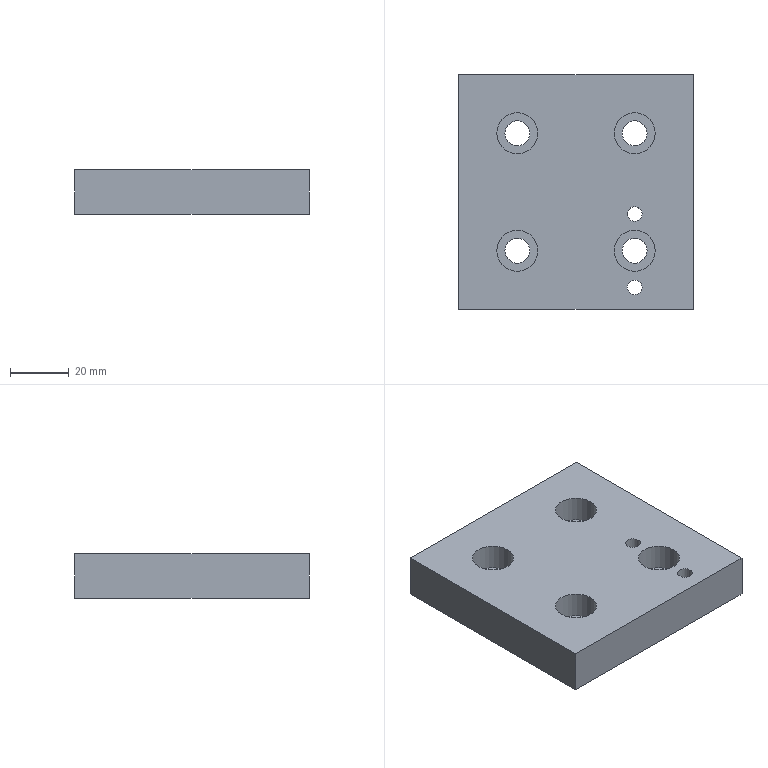Part | STEP file | 1 solid | 20 faces | box 80 x 80 x 15 mm | volume 88507 mm3 | plane 10 | cylinder 10 | commonest cylinder face diameters 8.5 x4 14 x4 5 x2
STEP:
#1=CARTESIAN_POINT('',(0.,0.,0.));
#2=DIRECTION('',(0.,0.,1.));
#3=DIRECTION('',(1.,0.,0.));
#4=AXIS2_PLACEMENT_3D('',#1,#2,#3);
#5=CARTESIAN_POINT('',(-5.75,-35.432,0.));
#6=VERTEX_POINT('',#5);
#7=CARTESIAN_POINT('',(-10.,-35.432,0.));
#8=DIRECTION('',(0.,0.,-1.));
#9=DIRECTION('',(1.,0.,0.));
#10=AXIS2_PLACEMENT_3D('',#7,#8,#9);
#11=CIRCLE('',#10,4.25);
#12=CARTESIAN_POINT('',(0.,0.,0.));
#13=DIRECTION('',(0.,0.,1.));
#14=DIRECTION('',(1.,0.,0.));
#15=AXIS2_PLACEMENT_3D('',#12,#13,#14);
#16=PLANE('',#15);
#17=CARTESIAN_POINT('',(-5.75,-35.432));
#18=CARTESIAN_POINT('',(-5.75,-42.793));
#19=CARTESIAN_POINT('',(-12.125,-39.113));
#20=CARTESIAN_POINT('',(-18.5,-35.432));
#21=CARTESIAN_POINT('',(-12.125,-31.751));
#22=CARTESIAN_POINT('',(-5.75,-28.071));
#23=CARTESIAN_POINT('',(-5.75,-35.432));
#24=(BOUNDED_CURVE()B_SPLINE_CURVE(2,(#17,#18,#19,#20,#21,#22,#23),.UNSPECIFIED.,.T.,.F.)B_SPLINE_CURVE_WITH_KNOTS((1,2,2,2,2,1),(-2.094,0.,2.094,4.189,6.283,8.378),.UNSPECIFIED.)CURVE()GEOMETRIC_REPRESENTATION_ITEM()RATIONAL_B_SPLINE_CURVE((1.,0.5,1.,0.5,1.,0.5,1.))REPRESENTATION_ITEM(''));
#25=(GEOMETRIC_REPRESENTATION_CONTEXT(2)PARAMETRIC_REPRESENTATION_CONTEXT()REPRESENTATION_CONTEXT('',''));
#26=DEFINITIONAL_REPRESENTATION('',(#24),#25);
#27=PCURVE('',#16,#26);
#28=CARTESIAN_POINT('',(-10.,-35.432,15.));
#29=DIRECTION('',(0.,0.,1.));
#30=DIRECTION('',(1.,0.,0.));
#31=AXIS2_PLACEMENT_3D('',#28,#29,#30);
#32=CYLINDRICAL_SURFACE('',#31,4.25);
#33=CARTESIAN_POINT('',(6.283,-15.));
#34=DIRECTION('',(-1.,0.));
#35=VECTOR('',#34,1.);
#36=LINE('',#33,#35);
#37=(GEOMETRIC_REPRESENTATION_CONTEXT(2)PARAMETRIC_REPRESENTATION_CONTEXT()REPRESENTATION_CONTEXT('',''));
#38=DEFINITIONAL_REPRESENTATION('',(#36),#37);
#39=PCURVE('',#32,#38);
#40=SURFACE_CURVE('',#11,(#27,#39),.PCURVE_S1.);
#41=EDGE_CURVE('',#6,#6,#40,.T.);
#42=ORIENTED_EDGE('',*,*,#41,.F.);
#43=EDGE_LOOP('',(#42));
#44=FACE_BOUND('',#43,.T.);
#45=CARTESIAN_POINT('',(-45.75,-35.432,0.));
#46=VERTEX_POINT('',#45);
#47=CARTESIAN_POINT('',(-50.,-35.432,0.));
#48=DIRECTION('',(0.,0.,-1.));
#49=DIRECTION('',(1.,0.,0.));
#50=AXIS2_PLACEMENT_3D('',#47,#48,#49);
#51=CIRCLE('',#50,4.25);
#52=CARTESIAN_POINT('',(-45.75,-35.432));
#53=CARTESIAN_POINT('',(-45.75,-42.793));
#54=CARTESIAN_POINT('',(-52.125,-39.113));
#55=CARTESIAN_POINT('',(-58.5,-35.432));
#56=CARTESIAN_POINT('',(-52.125,-31.751));
#57=CARTESIAN_POINT('',(-45.75,-28.071));
#58=CARTESIAN_POINT('',(-45.75,-35.432));
#59=(BOUNDED_CURVE()B_SPLINE_CURVE(2,(#52,#53,#54,#55,#56,#57,#58),.UNSPECIFIED.,.T.,.F.)B_SPLINE_CURVE_WITH_KNOTS((1,2,2,2,2,1),(-2.094,0.,2.094,4.189,6.283,8.378),.UNSPECIFIED.)CURVE()GEOMETRIC_REPRESENTATION_ITEM()RATIONAL_B_SPLINE_CURVE((1.,0.5,1.,0.5,1.,0.5,1.))REPRESENTATION_ITEM(''));
#60=(GEOMETRIC_REPRESENTATION_CONTEXT(2)PARAMETRIC_REPRESENTATION_CONTEXT()REPRESENTATION_CONTEXT('',''));
#61=DEFINITIONAL_REPRESENTATION('',(#59),#60);
#62=PCURVE('',#16,#61);
#63=CARTESIAN_POINT('',(-50.,-35.432,15.));
#64=DIRECTION('',(0.,0.,1.));
#65=DIRECTION('',(1.,0.,0.));
#66=AXIS2_PLACEMENT_3D('',#63,#64,#65);
#67=CYLINDRICAL_SURFACE('',#66,4.25);
#68=CARTESIAN_POINT('',(6.283,-15.));
#69=DIRECTION('',(-1.,0.));
#70=VECTOR('',#69,1.);
#71=LINE('',#68,#70);
#72=(GEOMETRIC_REPRESENTATION_CONTEXT(2)PARAMETRIC_REPRESENTATION_CONTEXT()REPRESENTATION_CONTEXT('',''));
#73=DEFINITIONAL_REPRESENTATION('',(#71),#72);
#74=PCURVE('',#67,#73);
#75=SURFACE_CURVE('',#51,(#62,#74),.PCURVE_S1.);
#76=EDGE_CURVE('',#46,#46,#75,.T.);
#77=ORIENTED_EDGE('',*,*,#76,.F.);
#78=EDGE_LOOP('',(#77));
#79=FACE_BOUND('',#78,.T.);
#80=CARTESIAN_POINT('',(-45.75,4.568,0.));
#81=VERTEX_POINT('',#80);
#82=CARTESIAN_POINT('',(-50.,4.568,0.));
#83=DIRECTION('',(0.,0.,-1.));
#84=DIRECTION('',(1.,0.,0.));
#85=AXIS2_PLACEMENT_3D('',#82,#83,#84);
#86=CIRCLE('',#85,4.25);
#87=CARTESIAN_POINT('',(-45.75,4.568));
#88=CARTESIAN_POINT('',(-45.75,-2.793));
#89=CARTESIAN_POINT('',(-52.125,0.8873));
#90=CARTESIAN_POINT('',(-58.5,4.568));
#91=CARTESIAN_POINT('',(-52.125,8.249));
#92=CARTESIAN_POINT('',(-45.75,11.929));
#93=CARTESIAN_POINT('',(-45.75,4.568));
#94=(BOUNDED_CURVE()B_SPLINE_CURVE(2,(#87,#88,#89,#90,#91,#92,#93),.UNSPECIFIED.,.T.,.F.)B_SPLINE_CURVE_WITH_KNOTS((1,2,2,2,2,1),(-2.094,0.,2.094,4.189,6.283,8.378),.UNSPECIFIED.)CURVE()GEOMETRIC_REPRESENTATION_ITEM()RATIONAL_B_SPLINE_CURVE((1.,0.5,1.,0.5,1.,0.5,1.))REPRESENTATION_ITEM(''));
#95=(GEOMETRIC_REPRESENTATION_CONTEXT(2)PARAMETRIC_REPRESENTATION_CONTEXT()REPRESENTATION_CONTEXT('',''));
#96=DEFINITIONAL_REPRESENTATION('',(#94),#95);
#97=PCURVE('',#16,#96);
#98=CARTESIAN_POINT('',(-50.,4.568,15.));
#99=DIRECTION('',(0.,0.,1.));
#100=DIRECTION('',(1.,0.,0.));
#101=AXIS2_PLACEMENT_3D('',#98,#99,#100);
#102=CYLINDRICAL_SURFACE('',#101,4.25);
#103=CARTESIAN_POINT('',(6.283,-15.));
#104=DIRECTION('',(-1.,0.));
#105=VECTOR('',#104,1.);
#106=LINE('',#103,#105);
#107=(GEOMETRIC_REPRESENTATION_CONTEXT(2)PARAMETRIC_REPRESENTATION_CONTEXT()REPRESENTATION_CONTEXT('',''));
#108=DEFINITIONAL_REPRESENTATION('',(#106),#107);
#109=PCURVE('',#102,#108);
#110=SURFACE_CURVE('',#86,(#97,#109),.PCURVE_S1.);
#111=EDGE_CURVE('',#81,#81,#110,.T.);
#112=ORIENTED_EDGE('',*,*,#111,.F.);
#113=EDGE_LOOP('',(#112));
#114=FACE_BOUND('',#113,.T.);
#115=CARTESIAN_POINT('',(-5.75,4.568,0.));
#116=VERTEX_POINT('',#115);
#117=CARTESIAN_POINT('',(-10.,4.568,0.));
#118=DIRECTION('',(0.,0.,-1.));
#119=DIRECTION('',(1.,0.,0.));
#120=AXIS2_PLACEMENT_3D('',#117,#118,#119);
#121=CIRCLE('',#120,4.25);
#122=CARTESIAN_POINT('',(-5.75,4.568));
#123=CARTESIAN_POINT('',(-5.75,-2.793));
#124=CARTESIAN_POINT('',(-12.125,0.8873));
#125=CARTESIAN_POINT('',(-18.5,4.568));
#126=CARTESIAN_POINT('',(-12.125,8.249));
#127=CARTESIAN_POINT('',(-5.75,11.929));
#128=CARTESIAN_POINT('',(-5.75,4.568));
#129=(BOUNDED_CURVE()B_SPLINE_CURVE(2,(#122,#123,#124,#125,#126,#127,#128),.UNSPECIFIED.,.T.,.F.)B_SPLINE_CURVE_WITH_KNOTS((1,2,2,2,2,1),(-2.094,0.,2.094,4.189,6.283,8.378),.UNSPECIFIED.)CURVE()GEOMETRIC_REPRESENTATION_ITEM()RATIONAL_B_SPLINE_CURVE((1.,0.5,1.,0.5,1.,0.5,1.))REPRESENTATION_ITEM(''));
#130=(GEOMETRIC_REPRESENTATION_CONTEXT(2)PARAMETRIC_REPRESENTATION_CONTEXT()REPRESENTATION_CONTEXT('',''));
#131=DEFINITIONAL_REPRESENTATION('',(#129),#130);
#132=PCURVE('',#16,#131);
#133=CARTESIAN_POINT('',(-10.,4.568,15.));
#134=DIRECTION('',(0.,0.,1.));
#135=DIRECTION('',(1.,0.,0.));
#136=AXIS2_PLACEMENT_3D('',#133,#134,#135);
#137=CYLINDRICAL_SURFACE('',#136,4.25);
#138=CARTESIAN_POINT('',(6.283,-15.));
#139=DIRECTION('',(-1.,0.));
#140=VECTOR('',#139,1.);
#141=LINE('',#138,#140);
#142=(GEOMETRIC_REPRESENTATION_CONTEXT(2)PARAMETRIC_REPRESENTATION_CONTEXT()REPRESENTATION_CONTEXT('',''));
#143=DEFINITIONAL_REPRESENTATION('',(#141),#142);
#144=PCURVE('',#137,#143);
#145=SURFACE_CURVE('',#121,(#132,#144),.PCURVE_S1.);
#146=EDGE_CURVE('',#116,#116,#145,.T.);
#147=ORIENTED_EDGE('',*,*,#146,.F.);
#148=EDGE_LOOP('',(#147));
#149=FACE_BOUND('',#148,.T.);
#150=CARTESIAN_POINT('',(-7.5,-47.932,0.));
#151=VERTEX_POINT('',#150);
#152=CARTESIAN_POINT('',(-10.,-47.932,0.));
#153=DIRECTION('',(0.,0.,-1.));
#154=DIRECTION('',(1.,0.,0.));
#155=AXIS2_PLACEMENT_3D('',#152,#153,#154);
#156=CIRCLE('',#155,2.5);
#157=CARTESIAN_POINT('',(-7.5,-47.932));
#158=CARTESIAN_POINT('',(-7.5,-52.262));
#159=CARTESIAN_POINT('',(-11.25,-50.097));
#160=CARTESIAN_POINT('',(-15.,-47.932));
#161=CARTESIAN_POINT('',(-11.25,-45.767));
#162=CARTESIAN_POINT('',(-7.5,-43.602));
#163=CARTESIAN_POINT('',(-7.5,-47.932));
#164=(BOUNDED_CURVE()B_SPLINE_CURVE(2,(#157,#158,#159,#160,#161,#162,#163),.UNSPECIFIED.,.T.,.F.)B_SPLINE_CURVE_WITH_KNOTS((1,2,2,2,2,1),(-2.094,0.,2.094,4.189,6.283,8.378),.UNSPECIFIED.)CURVE()GEOMETRIC_REPRESENTATION_ITEM()RATIONAL_B_SPLINE_CURVE((1.,0.5,1.,0.5,1.,0.5,1.))REPRESENTATION_ITEM(''));
#165=(GEOMETRIC_REPRESENTATION_CONTEXT(2)PARAMETRIC_REPRESENTATION_CONTEXT()REPRESENTATION_CONTEXT('',''));
#166=DEFINITIONAL_REPRESENTATION('',(#164),#165);
#167=PCURVE('',#16,#166);
#168=CARTESIAN_POINT('',(-10.,-47.932,15.));
#169=DIRECTION('',(0.,0.,1.));
#170=DIRECTION('',(1.,0.,0.));
#171=AXIS2_PLACEMENT_3D('',#168,#169,#170);
#172=CYLINDRICAL_SURFACE('',#171,2.5);
#173=CARTESIAN_POINT('',(6.283,-15.));
#174=DIRECTION('',(-1.,0.));
#175=VECTOR('',#174,1.);
#176=LINE('',#173,#175);
#177=(GEOMETRIC_REPRESENTATION_CONTEXT(2)PARAMETRIC_REPRESENTATION_CONTEXT()REPRESENTATION_CONTEXT('',''));
#178=DEFINITIONAL_REPRESENTATION('',(#176),#177);
#179=PCURVE('',#172,#178);
#180=SURFACE_CURVE('',#156,(#167,#179),.PCURVE_S1.);
#181=EDGE_CURVE('',#151,#151,#180,.T.);
#182=ORIENTED_EDGE('',*,*,#181,.F.);
#183=EDGE_LOOP('',(#182));
#184=FACE_BOUND('',#183,.T.);
#185=CARTESIAN_POINT('',(-7.5,-22.932,0.));
#186=VERTEX_POINT('',#185);
#187=CARTESIAN_POINT('',(-10.,-22.932,0.));
#188=DIRECTION('',(0.,0.,-1.));
#189=DIRECTION('',(1.,0.,0.));
#190=AXIS2_PLACEMENT_3D('',#187,#188,#189);
#191=CIRCLE('',#190,2.5);
#192=CARTESIAN_POINT('',(-7.5,-22.932));
#193=CARTESIAN_POINT('',(-7.5,-27.262));
#194=CARTESIAN_POINT('',(-11.25,-25.097));
#195=CARTESIAN_POINT('',(-15.,-22.932));
#196=CARTESIAN_POINT('',(-11.25,-20.767));
#197=CARTESIAN_POINT('',(-7.5,-18.602));
#198=CARTESIAN_POINT('',(-7.5,-22.932));
#199=(BOUNDED_CURVE()B_SPLINE_CURVE(2,(#192,#193,#194,#195,#196,#197,#198),.UNSPECIFIED.,.T.,.F.)B_SPLINE_CURVE_WITH_KNOTS((1,2,2,2,2,1),(-2.094,0.,2.094,4.189,6.283,8.378),.UNSPECIFIED.)CURVE()GEOMETRIC_REPRESENTATION_ITEM()RATIONAL_B_SPLINE_CURVE((1.,0.5,1.,0.5,1.,0.5,1.))REPRESENTATION_ITEM(''));
#200=(GEOMETRIC_REPRESENTATION_CONTEXT(2)PARAMETRIC_REPRESENTATION_CONTEXT()REPRESENTATION_CONTEXT('',''));
#201=DEFINITIONAL_REPRESENTATION('',(#199),#200);
#202=PCURVE('',#16,#201);
#203=CARTESIAN_POINT('',(-10.,-22.932,15.));
#204=DIRECTION('',(0.,0.,1.));
#205=DIRECTION('',(1.,0.,0.));
#206=AXIS2_PLACEMENT_3D('',#203,#204,#205);
#207=CYLINDRICAL_SURFACE('',#206,2.5);
#208=CARTESIAN_POINT('',(6.283,-15.));
#209=DIRECTION('',(-1.,0.));
#210=VECTOR('',#209,1.);
#211=LINE('',#208,#210);
#212=(GEOMETRIC_REPRESENTATION_CONTEXT(2)PARAMETRIC_REPRESENTATION_CONTEXT()REPRESENTATION_CONTEXT('',''));
#213=DEFINITIONAL_REPRESENTATION('',(#211),#212);
#214=PCURVE('',#207,#213);
#215=SURFACE_CURVE('',#191,(#202,#214),.PCURVE_S1.);
#216=EDGE_CURVE('',#186,#186,#215,.T.);
#217=ORIENTED_EDGE('',*,*,#216,.F.);
#218=EDGE_LOOP('',(#217));
#219=FACE_BOUND('',#218,.T.);
#220=CARTESIAN_POINT('',(10.,24.568,0.));
#221=VERTEX_POINT('',#220);
#222=CARTESIAN_POINT('',(-70.,24.568,0.));
#223=VERTEX_POINT('',#222);
#224=CARTESIAN_POINT('',(0.,24.568,0.));
#225=DIRECTION('',(-1.,0.,0.));
#226=VECTOR('',#225,1.);
#227=LINE('',#224,#226);
#228=CARTESIAN_POINT('',(0.,24.568));
#229=DIRECTION('',(-1.,0.));
#230=VECTOR('',#229,1.);
#231=LINE('',#228,#230);
#232=(GEOMETRIC_REPRESENTATION_CONTEXT(2)PARAMETRIC_REPRESENTATION_CONTEXT()REPRESENTATION_CONTEXT('',''));
#233=DEFINITIONAL_REPRESENTATION('',(#231),#232);
#234=PCURVE('',#16,#233);
#235=CARTESIAN_POINT('',(-70.,24.568,15.));
#236=DIRECTION('',(0.,-1.,0.));
#237=DIRECTION('',(0.,0.,-1.));
#238=AXIS2_PLACEMENT_3D('',#235,#236,#237);
#239=PLANE('',#238);
#240=CARTESIAN_POINT('',(15.,70.));
#241=DIRECTION('',(0.,-1.));
#242=VECTOR('',#241,1.);
#243=LINE('',#240,#242);
#244=(GEOMETRIC_REPRESENTATION_CONTEXT(2)PARAMETRIC_REPRESENTATION_CONTEXT()REPRESENTATION_CONTEXT('',''));
#245=DEFINITIONAL_REPRESENTATION('',(#243),#244);
#246=PCURVE('',#239,#245);
#247=SURFACE_CURVE('',#227,(#234,#246),.PCURVE_S1.);
#248=EDGE_CURVE('',#221,#223,#247,.T.);
#249=ORIENTED_EDGE('',*,*,#248,.F.);
#250=CARTESIAN_POINT('',(10.,-55.432,0.));
#251=VERTEX_POINT('',#250);
#252=CARTESIAN_POINT('',(10.,0.,0.));
#253=DIRECTION('',(0.,1.,0.));
#254=VECTOR('',#253,1.);
#255=LINE('',#252,#254);
#256=CARTESIAN_POINT('',(10.,0.));
#257=DIRECTION('',(0.,1.));
#258=VECTOR('',#257,1.);
#259=LINE('',#256,#258);
#260=(GEOMETRIC_REPRESENTATION_CONTEXT(2)PARAMETRIC_REPRESENTATION_CONTEXT()REPRESENTATION_CONTEXT('',''));
#261=DEFINITIONAL_REPRESENTATION('',(#259),#260);
#262=PCURVE('',#16,#261);
#263=CARTESIAN_POINT('',(10.,24.568,15.));
#264=DIRECTION('',(-1.,0.,0.));
#265=DIRECTION('',(0.,-1.,0.));
#266=AXIS2_PLACEMENT_3D('',#263,#264,#265);
#267=PLANE('',#266);
#268=CARTESIAN_POINT('',(24.568,-15.));
#269=DIRECTION('',(-1.,0.));
#270=VECTOR('',#269,1.);
#271=LINE('',#268,#270);
#272=(GEOMETRIC_REPRESENTATION_CONTEXT(2)PARAMETRIC_REPRESENTATION_CONTEXT()REPRESENTATION_CONTEXT('',''));
#273=DEFINITIONAL_REPRESENTATION('',(#271),#272);
#274=PCURVE('',#267,#273);
#275=SURFACE_CURVE('',#255,(#262,#274),.PCURVE_S1.);
#276=EDGE_CURVE('',#251,#221,#275,.T.);
#277=ORIENTED_EDGE('',*,*,#276,.F.);
#278=CARTESIAN_POINT('',(-70.,-55.432,0.));
#279=VERTEX_POINT('',#278);
#280=CARTESIAN_POINT('',(0.,-55.432,0.));
#281=DIRECTION('',(1.,0.,0.));
#282=VECTOR('',#281,1.);
#283=LINE('',#280,#282);
#284=CARTESIAN_POINT('',(0.,-55.432));
#285=DIRECTION('',(1.,0.));
#286=VECTOR('',#285,1.);
#287=LINE('',#284,#286);
#288=(GEOMETRIC_REPRESENTATION_CONTEXT(2)PARAMETRIC_REPRESENTATION_CONTEXT()REPRESENTATION_CONTEXT('',''));
#289=DEFINITIONAL_REPRESENTATION('',(#287),#288);
#290=PCURVE('',#16,#289);
#291=CARTESIAN_POINT('',(-70.,-55.432,15.));
#292=DIRECTION('',(0.,1.,0.));
#293=DIRECTION('',(0.,0.,1.));
#294=AXIS2_PLACEMENT_3D('',#291,#292,#293);
#295=PLANE('',#294);
#296=CARTESIAN_POINT('',(-15.,70.));
#297=DIRECTION('',(0.,1.));
#298=VECTOR('',#297,1.);
#299=LINE('',#296,#298);
#300=(GEOMETRIC_REPRESENTATION_CONTEXT(2)PARAMETRIC_REPRESENTATION_CONTEXT()REPRESENTATION_CONTEXT('',''));
#301=DEFINITIONAL_REPRESENTATION('',(#299),#300);
#302=PCURVE('',#295,#301);
#303=SURFACE_CURVE('',#283,(#290,#302),.PCURVE_S1.);
#304=EDGE_CURVE('',#279,#251,#303,.T.);
#305=ORIENTED_EDGE('',*,*,#304,.F.);
#306=CARTESIAN_POINT('',(-70.,0.,0.));
#307=DIRECTION('',(0.,-1.,0.));
#308=VECTOR('',#307,1.);
#309=LINE('',#306,#308);
#310=CARTESIAN_POINT('',(-70.,0.));
#311=DIRECTION('',(0.,-1.));
#312=VECTOR('',#311,1.);
#313=LINE('',#310,#312);
#314=(GEOMETRIC_REPRESENTATION_CONTEXT(2)PARAMETRIC_REPRESENTATION_CONTEXT()REPRESENTATION_CONTEXT('',''));
#315=DEFINITIONAL_REPRESENTATION('',(#313),#314);
#316=PCURVE('',#16,#315);
#317=CARTESIAN_POINT('',(-70.,24.568,15.));
#318=DIRECTION('',(1.,0.,0.));
#319=DIRECTION('',(0.,0.,-1.));
#320=AXIS2_PLACEMENT_3D('',#317,#318,#319);
#321=PLANE('',#320);
#322=CARTESIAN_POINT('',(15.,-24.568));
#323=DIRECTION('',(0.,-1.));
#324=VECTOR('',#323,1.);
#325=LINE('',#322,#324);
#326=(GEOMETRIC_REPRESENTATION_CONTEXT(2)PARAMETRIC_REPRESENTATION_CONTEXT()REPRESENTATION_CONTEXT('',''));
#327=DEFINITIONAL_REPRESENTATION('',(#325),#326);
#328=PCURVE('',#321,#327);
#329=SURFACE_CURVE('',#309,(#316,#328),.PCURVE_S1.);
#330=EDGE_CURVE('',#223,#279,#329,.T.);
#331=ORIENTED_EDGE('',*,*,#330,.F.);
#332=EDGE_LOOP('',(#249,#277,#305,#331));
#333=FACE_BOUND('',#332,.T.);
#334=ADVANCED_FACE('',(#44,#79,#114,#149,#184,#219,#333),#16,.F.);
#335=ORIENTED_EDGE('',*,*,#41,.F.);
#336=CARTESIAN_POINT('',(-5.75,-35.432,6.));
#337=VERTEX_POINT('',#336);
#338=CARTESIAN_POINT('',(-5.75,-35.432,0.));
#339=CARTESIAN_POINT('',(-5.75,-35.432,6.));
#340=B_SPLINE_CURVE_WITH_KNOTS('',1,(#338,#339),.UNSPECIFIED.,.F.,.F.,(2,2),(-15.,-9.),.PIECEWISE_BEZIER_KNOTS.);
#341=CARTESIAN_POINT('',(6.283,0.));
#342=DIRECTION('',(0.,1.));
#343=VECTOR('',#342,1.);
#344=LINE('',#341,#343);
#345=(GEOMETRIC_REPRESENTATION_CONTEXT(2)PARAMETRIC_REPRESENTATION_CONTEXT()REPRESENTATION_CONTEXT('',''));
#346=DEFINITIONAL_REPRESENTATION('',(#344),#345);
#347=PCURVE('',#32,#346);
#348=CARTESIAN_POINT('',(0.,0.));
#349=DIRECTION('',(0.,1.));
#350=VECTOR('',#349,1.);
#351=LINE('',#348,#350);
#352=(GEOMETRIC_REPRESENTATION_CONTEXT(2)PARAMETRIC_REPRESENTATION_CONTEXT()REPRESENTATION_CONTEXT('',''));
#353=DEFINITIONAL_REPRESENTATION('',(#351),#352);
#354=PCURVE('',#32,#353);
#355=SEAM_CURVE('',#340,(#347,#354),.PCURVE_S1.);
#356=EDGE_CURVE('',#6,#337,#355,.T.);
#357=ORIENTED_EDGE('',*,*,#356,.T.);
#358=CARTESIAN_POINT('',(-10.,-35.432,6.));
#359=DIRECTION('',(0.,0.,-1.));
#360=DIRECTION('',(1.,0.,0.));
#361=AXIS2_PLACEMENT_3D('',#358,#359,#360);
#362=CIRCLE('',#361,4.25);
#363=CARTESIAN_POINT('',(6.283,-9.));
#364=DIRECTION('',(-1.,0.));
#365=VECTOR('',#364,1.);
#366=LINE('',#363,#365);
#367=(GEOMETRIC_REPRESENTATION_CONTEXT(2)PARAMETRIC_REPRESENTATION_CONTEXT()REPRESENTATION_CONTEXT('',''));
#368=DEFINITIONAL_REPRESENTATION('',(#366),#367);
#369=PCURVE('',#32,#368);
#370=CARTESIAN_POINT('',(-5.75,-35.432,6.));
#371=DIRECTION('',(0.,0.,-1.));
#372=DIRECTION('',(-1.,0.,0.));
#373=AXIS2_PLACEMENT_3D('',#370,#371,#372);
#374=PLANE('',#373);
#375=CARTESIAN_POINT('',(4.25,0.));
#376=DIRECTION('',(-1.,0.));
#377=AXIS2_PLACEMENT_2D('',#375,#376);
#378=CIRCLE('',#377,4.25);
#379=(GEOMETRIC_REPRESENTATION_CONTEXT(2)PARAMETRIC_REPRESENTATION_CONTEXT()REPRESENTATION_CONTEXT('',''));
#380=DEFINITIONAL_REPRESENTATION('',(#378),#379);
#381=PCURVE('',#374,#380);
#382=SURFACE_CURVE('',#362,(#369,#381),.PCURVE_S1.);
#383=EDGE_CURVE('',#337,#337,#382,.T.);
#384=ORIENTED_EDGE('',*,*,#383,.T.);
#385=ORIENTED_EDGE('',*,*,#356,.F.);
#386=EDGE_LOOP('',(#335,#357,#384,#385));
#387=FACE_BOUND('',#386,.F.);
#388=ADVANCED_FACE('',(#387),#32,.F.);
#389=ORIENTED_EDGE('',*,*,#76,.F.);
#390=CARTESIAN_POINT('',(-45.75,-35.432,6.));
#391=VERTEX_POINT('',#390);
#392=CARTESIAN_POINT('',(-45.75,-35.432,0.));
#393=CARTESIAN_POINT('',(-45.75,-35.432,6.));
#394=B_SPLINE_CURVE_WITH_KNOTS('',1,(#392,#393),.UNSPECIFIED.,.F.,.F.,(2,2),(-15.,-9.),.PIECEWISE_BEZIER_KNOTS.);
#395=CARTESIAN_POINT('',(6.283,0.));
#396=DIRECTION('',(0.,1.));
#397=VECTOR('',#396,1.);
#398=LINE('',#395,#397);
#399=(GEOMETRIC_REPRESENTATION_CONTEXT(2)PARAMETRIC_REPRESENTATION_CONTEXT()REPRESENTATION_CONTEXT('',''));
#400=DEFINITIONAL_REPRESENTATION('',(#398),#399);
#401=PCURVE('',#67,#400);
#402=CARTESIAN_POINT('',(0.,0.));
#403=DIRECTION('',(0.,1.));
#404=VECTOR('',#403,1.);
#405=LINE('',#402,#404);
#406=(GEOMETRIC_REPRESENTATION_CONTEXT(2)PARAMETRIC_REPRESENTATION_CONTEXT()REPRESENTATION_CONTEXT('',''));
#407=DEFINITIONAL_REPRESENTATION('',(#405),#406);
#408=PCURVE('',#67,#407);
#409=SEAM_CURVE('',#394,(#401,#408),.PCURVE_S1.);
#410=EDGE_CURVE('',#46,#391,#409,.T.);
#411=ORIENTED_EDGE('',*,*,#410,.T.);
#412=CARTESIAN_POINT('',(-50.,-35.432,6.));
#413=DIRECTION('',(0.,0.,-1.));
#414=DIRECTION('',(1.,0.,0.));
#415=AXIS2_PLACEMENT_3D('',#412,#413,#414);
#416=CIRCLE('',#415,4.25);
#417=CARTESIAN_POINT('',(6.283,-9.));
#418=DIRECTION('',(-1.,0.));
#419=VECTOR('',#418,1.);
#420=LINE('',#417,#419);
#421=(GEOMETRIC_REPRESENTATION_CONTEXT(2)PARAMETRIC_REPRESENTATION_CONTEXT()REPRESENTATION_CONTEXT('',''));
#422=DEFINITIONAL_REPRESENTATION('',(#420),#421);
#423=PCURVE('',#67,#422);
#424=CARTESIAN_POINT('',(-45.75,-35.432,6.));
#425=DIRECTION('',(0.,0.,-1.));
#426=DIRECTION('',(-1.,0.,0.));
#427=AXIS2_PLACEMENT_3D('',#424,#425,#426);
#428=PLANE('',#427);
#429=CARTESIAN_POINT('',(4.25,0.));
#430=DIRECTION('',(-1.,0.));
#431=AXIS2_PLACEMENT_2D('',#429,#430);
#432=CIRCLE('',#431,4.25);
#433=(GEOMETRIC_REPRESENTATION_CONTEXT(2)PARAMETRIC_REPRESENTATION_CONTEXT()REPRESENTATION_CONTEXT('',''));
#434=DEFINITIONAL_REPRESENTATION('',(#432),#433);
#435=PCURVE('',#428,#434);
#436=SURFACE_CURVE('',#416,(#423,#435),.PCURVE_S1.);
#437=EDGE_CURVE('',#391,#391,#436,.T.);
#438=ORIENTED_EDGE('',*,*,#437,.T.);
#439=ORIENTED_EDGE('',*,*,#410,.F.);
#440=EDGE_LOOP('',(#389,#411,#438,#439));
#441=FACE_BOUND('',#440,.F.);
#442=ADVANCED_FACE('',(#441),#67,.F.);
#443=ORIENTED_EDGE('',*,*,#111,.F.);
#444=CARTESIAN_POINT('',(-45.75,4.568,6.));
#445=VERTEX_POINT('',#444);
#446=CARTESIAN_POINT('',(-45.75,4.568,0.));
#447=CARTESIAN_POINT('',(-45.75,4.568,6.));
#448=B_SPLINE_CURVE_WITH_KNOTS('',1,(#446,#447),.UNSPECIFIED.,.F.,.F.,(2,2),(-15.,-9.),.PIECEWISE_BEZIER_KNOTS.);
#449=CARTESIAN_POINT('',(6.283,0.));
#450=DIRECTION('',(0.,1.));
#451=VECTOR('',#450,1.);
#452=LINE('',#449,#451);
#453=(GEOMETRIC_REPRESENTATION_CONTEXT(2)PARAMETRIC_REPRESENTATION_CONTEXT()REPRESENTATION_CONTEXT('',''));
#454=DEFINITIONAL_REPRESENTATION('',(#452),#453);
#455=PCURVE('',#102,#454);
#456=CARTESIAN_POINT('',(0.,0.));
#457=DIRECTION('',(0.,1.));
#458=VECTOR('',#457,1.);
#459=LINE('',#456,#458);
#460=(GEOMETRIC_REPRESENTATION_CONTEXT(2)PARAMETRIC_REPRESENTATION_CONTEXT()REPRESENTATION_CONTEXT('',''));
#461=DEFINITIONAL_REPRESENTATION('',(#459),#460);
#462=PCURVE('',#102,#461);
#463=SEAM_CURVE('',#448,(#455,#462),.PCURVE_S1.);
#464=EDGE_CURVE('',#81,#445,#463,.T.);
#465=ORIENTED_EDGE('',*,*,#464,.T.);
#466=CARTESIAN_POINT('',(-50.,4.568,6.));
#467=DIRECTION('',(0.,0.,-1.));
#468=DIRECTION('',(1.,0.,0.));
#469=AXIS2_PLACEMENT_3D('',#466,#467,#468);
#470=CIRCLE('',#469,4.25);
#471=CARTESIAN_POINT('',(6.283,-9.));
#472=DIRECTION('',(-1.,0.));
#473=VECTOR('',#472,1.);
#474=LINE('',#471,#473);
#475=(GEOMETRIC_REPRESENTATION_CONTEXT(2)PARAMETRIC_REPRESENTATION_CONTEXT()REPRESENTATION_CONTEXT('',''));
#476=DEFINITIONAL_REPRESENTATION('',(#474),#475);
#477=PCURVE('',#102,#476);
#478=CARTESIAN_POINT('',(-45.75,4.568,6.));
#479=DIRECTION('',(0.,0.,-1.));
#480=DIRECTION('',(-1.,0.,0.));
#481=AXIS2_PLACEMENT_3D('',#478,#479,#480);
#482=PLANE('',#481);
#483=CARTESIAN_POINT('',(4.25,0.));
#484=DIRECTION('',(-1.,0.));
#485=AXIS2_PLACEMENT_2D('',#483,#484);
#486=CIRCLE('',#485,4.25);
#487=(GEOMETRIC_REPRESENTATION_CONTEXT(2)PARAMETRIC_REPRESENTATION_CONTEXT()REPRESENTATION_CONTEXT('',''));
#488=DEFINITIONAL_REPRESENTATION('',(#486),#487);
#489=PCURVE('',#482,#488);
#490=SURFACE_CURVE('',#470,(#477,#489),.PCURVE_S1.);
#491=EDGE_CURVE('',#445,#445,#490,.T.);
#492=ORIENTED_EDGE('',*,*,#491,.T.);
#493=ORIENTED_EDGE('',*,*,#464,.F.);
#494=EDGE_LOOP('',(#443,#465,#492,#493));
#495=FACE_BOUND('',#494,.F.);
#496=ADVANCED_FACE('',(#495),#102,.F.);
#497=ORIENTED_EDGE('',*,*,#146,.F.);
#498=CARTESIAN_POINT('',(-5.75,4.568,6.));
#499=VERTEX_POINT('',#498);
#500=CARTESIAN_POINT('',(-5.75,4.568,0.));
#501=CARTESIAN_POINT('',(-5.75,4.568,6.));
#502=B_SPLINE_CURVE_WITH_KNOTS('',1,(#500,#501),.UNSPECIFIED.,.F.,.F.,(2,2),(-15.,-9.),.PIECEWISE_BEZIER_KNOTS.);
#503=CARTESIAN_POINT('',(6.283,0.));
#504=DIRECTION('',(0.,1.));
#505=VECTOR('',#504,1.);
#506=LINE('',#503,#505);
#507=(GEOMETRIC_REPRESENTATION_CONTEXT(2)PARAMETRIC_REPRESENTATION_CONTEXT()REPRESENTATION_CONTEXT('',''));
#508=DEFINITIONAL_REPRESENTATION('',(#506),#507);
#509=PCURVE('',#137,#508);
#510=CARTESIAN_POINT('',(0.,0.));
#511=DIRECTION('',(0.,1.));
#512=VECTOR('',#511,1.);
#513=LINE('',#510,#512);
#514=(GEOMETRIC_REPRESENTATION_CONTEXT(2)PARAMETRIC_REPRESENTATION_CONTEXT()REPRESENTATION_CONTEXT('',''));
#515=DEFINITIONAL_REPRESENTATION('',(#513),#514);
#516=PCURVE('',#137,#515);
#517=SEAM_CURVE('',#502,(#509,#516),.PCURVE_S1.);
#518=EDGE_CURVE('',#116,#499,#517,.T.);
#519=ORIENTED_EDGE('',*,*,#518,.T.);
#520=CARTESIAN_POINT('',(-10.,4.568,6.));
#521=DIRECTION('',(0.,0.,-1.));
#522=DIRECTION('',(1.,0.,0.));
#523=AXIS2_PLACEMENT_3D('',#520,#521,#522);
#524=CIRCLE('',#523,4.25);
#525=CARTESIAN_POINT('',(6.283,-9.));
#526=DIRECTION('',(-1.,0.));
#527=VECTOR('',#526,1.);
#528=LINE('',#525,#527);
#529=(GEOMETRIC_REPRESENTATION_CONTEXT(2)PARAMETRIC_REPRESENTATION_CONTEXT()REPRESENTATION_CONTEXT('',''));
#530=DEFINITIONAL_REPRESENTATION('',(#528),#529);
#531=PCURVE('',#137,#530);
#532=CARTESIAN_POINT('',(-5.75,4.568,6.));
#533=DIRECTION('',(0.,0.,-1.));
#534=DIRECTION('',(-1.,0.,0.));
#535=AXIS2_PLACEMENT_3D('',#532,#533,#534);
#536=PLANE('',#535);
#537=CARTESIAN_POINT('',(4.25,0.));
#538=DIRECTION('',(-1.,0.));
#539=AXIS2_PLACEMENT_2D('',#537,#538);
#540=CIRCLE('',#539,4.25);
#541=(GEOMETRIC_REPRESENTATION_CONTEXT(2)PARAMETRIC_REPRESENTATION_CONTEXT()REPRESENTATION_CONTEXT('',''));
#542=DEFINITIONAL_REPRESENTATION('',(#540),#541);
#543=PCURVE('',#536,#542);
#544=SURFACE_CURVE('',#524,(#531,#543),.PCURVE_S1.);
#545=EDGE_CURVE('',#499,#499,#544,.T.);
#546=ORIENTED_EDGE('',*,*,#545,.T.);
#547=ORIENTED_EDGE('',*,*,#518,.F.);
#548=EDGE_LOOP('',(#497,#519,#546,#547));
#549=FACE_BOUND('',#548,.F.);
#550=ADVANCED_FACE('',(#549),#137,.F.);
#551=ORIENTED_EDGE('',*,*,#181,.F.);
#552=CARTESIAN_POINT('',(-7.5,-47.932,15.));
#553=VERTEX_POINT('',#552);
#554=CARTESIAN_POINT('',(-7.5,-47.932,0.));
#555=CARTESIAN_POINT('',(-7.5,-47.932,15.));
#556=B_SPLINE_CURVE_WITH_KNOTS('',1,(#554,#555),.UNSPECIFIED.,.F.,.F.,(2,2),(-15.,0.),.PIECEWISE_BEZIER_KNOTS.);
#557=CARTESIAN_POINT('',(6.283,0.));
#558=DIRECTION('',(0.,1.));
#559=VECTOR('',#558,1.);
#560=LINE('',#557,#559);
#561=(GEOMETRIC_REPRESENTATION_CONTEXT(2)PARAMETRIC_REPRESENTATION_CONTEXT()REPRESENTATION_CONTEXT('',''));
#562=DEFINITIONAL_REPRESENTATION('',(#560),#561);
#563=PCURVE('',#172,#562);
#564=CARTESIAN_POINT('',(0.,0.));
#565=DIRECTION('',(0.,1.));
#566=VECTOR('',#565,1.);
#567=LINE('',#564,#566);
#568=(GEOMETRIC_REPRESENTATION_CONTEXT(2)PARAMETRIC_REPRESENTATION_CONTEXT()REPRESENTATION_CONTEXT('',''));
#569=DEFINITIONAL_REPRESENTATION('',(#567),#568);
#570=PCURVE('',#172,#569);
#571=SEAM_CURVE('',#556,(#563,#570),.PCURVE_S1.);
#572=EDGE_CURVE('',#151,#553,#571,.T.);
#573=ORIENTED_EDGE('',*,*,#572,.T.);
#574=CARTESIAN_POINT('',(-10.,-47.932,15.));
#575=DIRECTION('',(0.,0.,-1.));
#576=DIRECTION('',(1.,0.,0.));
#577=AXIS2_PLACEMENT_3D('',#574,#575,#576);
#578=CIRCLE('',#577,2.5);
#579=CARTESIAN_POINT('',(6.283,0.));
#580=DIRECTION('',(-1.,0.));
#581=VECTOR('',#580,1.);
#582=LINE('',#579,#581);
#583=(GEOMETRIC_REPRESENTATION_CONTEXT(2)PARAMETRIC_REPRESENTATION_CONTEXT()REPRESENTATION_CONTEXT('',''));
#584=DEFINITIONAL_REPRESENTATION('',(#582),#583);
#585=PCURVE('',#172,#584);
#586=CARTESIAN_POINT('',(0.,0.,15.));
#587=DIRECTION('',(0.,0.,1.));
#588=DIRECTION('',(1.,0.,0.));
#589=AXIS2_PLACEMENT_3D('',#586,#587,#588);
#590=PLANE('',#589);
#591=CARTESIAN_POINT('',(-7.5,-47.932));
#592=CARTESIAN_POINT('',(-7.5,-52.262));
#593=CARTESIAN_POINT('',(-11.25,-50.097));
#594=CARTESIAN_POINT('',(-15.,-47.932));
#595=CARTESIAN_POINT('',(-11.25,-45.767));
#596=CARTESIAN_POINT('',(-7.5,-43.602));
#597=CARTESIAN_POINT('',(-7.5,-47.932));
#598=(BOUNDED_CURVE()B_SPLINE_CURVE(2,(#591,#592,#593,#594,#595,#596,#597),.UNSPECIFIED.,.T.,.F.)B_SPLINE_CURVE_WITH_KNOTS((1,2,2,2,2,1),(-2.094,0.,2.094,4.189,6.283,8.378),.UNSPECIFIED.)CURVE()GEOMETRIC_REPRESENTATION_ITEM()RATIONAL_B_SPLINE_CURVE((1.,0.5,1.,0.5,1.,0.5,1.))REPRESENTATION_ITEM(''));
#599=(GEOMETRIC_REPRESENTATION_CONTEXT(2)PARAMETRIC_REPRESENTATION_CONTEXT()REPRESENTATION_CONTEXT('',''));
#600=DEFINITIONAL_REPRESENTATION('',(#598),#599);
#601=PCURVE('',#590,#600);
#602=SURFACE_CURVE('',#578,(#585,#601),.PCURVE_S1.);
#603=EDGE_CURVE('',#553,#553,#602,.T.);
#604=ORIENTED_EDGE('',*,*,#603,.T.);
#605=ORIENTED_EDGE('',*,*,#572,.F.);
#606=EDGE_LOOP('',(#551,#573,#604,#605));
#607=FACE_BOUND('',#606,.F.);
#608=ADVANCED_FACE('',(#607),#172,.F.);
#609=ORIENTED_EDGE('',*,*,#216,.F.);
#610=CARTESIAN_POINT('',(-7.5,-22.932,15.));
#611=VERTEX_POINT('',#610);
#612=CARTESIAN_POINT('',(-7.5,-22.932,0.));
#613=CARTESIAN_POINT('',(-7.5,-22.932,15.));
#614=B_SPLINE_CURVE_WITH_KNOTS('',1,(#612,#613),.UNSPECIFIED.,.F.,.F.,(2,2),(-15.,0.),.PIECEWISE_BEZIER_KNOTS.);
#615=CARTESIAN_POINT('',(6.283,0.));
#616=DIRECTION('',(0.,1.));
#617=VECTOR('',#616,1.);
#618=LINE('',#615,#617);
#619=(GEOMETRIC_REPRESENTATION_CONTEXT(2)PARAMETRIC_REPRESENTATION_CONTEXT()REPRESENTATION_CONTEXT('',''));
#620=DEFINITIONAL_REPRESENTATION('',(#618),#619);
#621=PCURVE('',#207,#620);
#622=CARTESIAN_POINT('',(0.,0.));
#623=DIRECTION('',(0.,1.));
#624=VECTOR('',#623,1.);
#625=LINE('',#622,#624);
#626=(GEOMETRIC_REPRESENTATION_CONTEXT(2)PARAMETRIC_REPRESENTATION_CONTEXT()REPRESENTATION_CONTEXT('',''));
#627=DEFINITIONAL_REPRESENTATION('',(#625),#626);
#628=PCURVE('',#207,#627);
#629=SEAM_CURVE('',#614,(#621,#628),.PCURVE_S1.);
#630=EDGE_CURVE('',#186,#611,#629,.T.);
#631=ORIENTED_EDGE('',*,*,#630,.T.);
#632=CARTESIAN_POINT('',(-10.,-22.932,15.));
#633=DIRECTION('',(0.,0.,-1.));
#634=DIRECTION('',(1.,0.,0.));
#635=AXIS2_PLACEMENT_3D('',#632,#633,#634);
#636=CIRCLE('',#635,2.5);
#637=CARTESIAN_POINT('',(6.283,0.));
#638=DIRECTION('',(-1.,0.));
#639=VECTOR('',#638,1.);
#640=LINE('',#637,#639);
#641=(GEOMETRIC_REPRESENTATION_CONTEXT(2)PARAMETRIC_REPRESENTATION_CONTEXT()REPRESENTATION_CONTEXT('',''));
#642=DEFINITIONAL_REPRESENTATION('',(#640),#641);
#643=PCURVE('',#207,#642);
#644=CARTESIAN_POINT('',(-7.5,-22.932));
#645=CARTESIAN_POINT('',(-7.5,-27.262));
#646=CARTESIAN_POINT('',(-11.25,-25.097));
#647=CARTESIAN_POINT('',(-15.,-22.932));
#648=CARTESIAN_POINT('',(-11.25,-20.767));
#649=CARTESIAN_POINT('',(-7.5,-18.602));
#650=CARTESIAN_POINT('',(-7.5,-22.932));
#651=(BOUNDED_CURVE()B_SPLINE_CURVE(2,(#644,#645,#646,#647,#648,#649,#650),.UNSPECIFIED.,.T.,.F.)B_SPLINE_CURVE_WITH_KNOTS((1,2,2,2,2,1),(-2.094,0.,2.094,4.189,6.283,8.378),.UNSPECIFIED.)CURVE()GEOMETRIC_REPRESENTATION_ITEM()RATIONAL_B_SPLINE_CURVE((1.,0.5,1.,0.5,1.,0.5,1.))REPRESENTATION_ITEM(''));
#652=(GEOMETRIC_REPRESENTATION_CONTEXT(2)PARAMETRIC_REPRESENTATION_CONTEXT()REPRESENTATION_CONTEXT('',''));
#653=DEFINITIONAL_REPRESENTATION('',(#651),#652);
#654=PCURVE('',#590,#653);
#655=SURFACE_CURVE('',#636,(#643,#654),.PCURVE_S1.);
#656=EDGE_CURVE('',#611,#611,#655,.T.);
#657=ORIENTED_EDGE('',*,*,#656,.T.);
#658=ORIENTED_EDGE('',*,*,#630,.F.);
#659=EDGE_LOOP('',(#609,#631,#657,#658));
#660=FACE_BOUND('',#659,.F.);
#661=ADVANCED_FACE('',(#660),#207,.F.);
#662=CARTESIAN_POINT('',(-70.,-55.432,15.));
#663=VERTEX_POINT('',#662);
#664=CARTESIAN_POINT('',(-70.,-55.432,15.));
#665=DIRECTION('',(0.,0.,-1.));
#666=VECTOR('',#665,1.);
#667=LINE('',#664,#666);
#668=CARTESIAN_POINT('',(0.,-80.));
#669=DIRECTION('',(1.,0.));
#670=VECTOR('',#669,1.);
#671=LINE('',#668,#670);
#672=(GEOMETRIC_REPRESENTATION_CONTEXT(2)PARAMETRIC_REPRESENTATION_CONTEXT()REPRESENTATION_CONTEXT('',''));
#673=DEFINITIONAL_REPRESENTATION('',(#671),#672);
#674=PCURVE('',#321,#673);
#675=CARTESIAN_POINT('',(0.,0.));
#676=DIRECTION('',(-1.,0.));
#677=VECTOR('',#676,1.);
#678=LINE('',#675,#677);
#679=(GEOMETRIC_REPRESENTATION_CONTEXT(2)PARAMETRIC_REPRESENTATION_CONTEXT()REPRESENTATION_CONTEXT('',''));
#680=DEFINITIONAL_REPRESENTATION('',(#678),#679);
#681=PCURVE('',#295,#680);
#682=SURFACE_CURVE('',#667,(#674,#681),.PCURVE_S1.);
#683=EDGE_CURVE('',#663,#279,#682,.T.);
#684=ORIENTED_EDGE('',*,*,#683,.F.);
#685=CARTESIAN_POINT('',(-70.,24.568,15.));
#686=VERTEX_POINT('',#685);
#687=CARTESIAN_POINT('',(-70.,24.568,15.));
#688=DIRECTION('',(0.,-1.,0.));
#689=VECTOR('',#688,1.);
#690=LINE('',#687,#689);
#691=CARTESIAN_POINT('',(0.,0.));
#692=DIRECTION('',(0.,-1.));
#693=VECTOR('',#692,1.);
#694=LINE('',#691,#693);
#695=(GEOMETRIC_REPRESENTATION_CONTEXT(2)PARAMETRIC_REPRESENTATION_CONTEXT()REPRESENTATION_CONTEXT('',''));
#696=DEFINITIONAL_REPRESENTATION('',(#694),#695);
#697=PCURVE('',#321,#696);
#698=CARTESIAN_POINT('',(-70.,24.568));
#699=DIRECTION('',(0.,-1.));
#700=VECTOR('',#699,1.);
#701=LINE('',#698,#700);
#702=(GEOMETRIC_REPRESENTATION_CONTEXT(2)PARAMETRIC_REPRESENTATION_CONTEXT()REPRESENTATION_CONTEXT('',''));
#703=DEFINITIONAL_REPRESENTATION('',(#701),#702);
#704=PCURVE('',#590,#703);
#705=SURFACE_CURVE('',#690,(#697,#704),.PCURVE_S1.);
#706=EDGE_CURVE('',#686,#663,#705,.T.);
#707=ORIENTED_EDGE('',*,*,#706,.F.);
#708=CARTESIAN_POINT('',(-70.,24.568,15.));
#709=DIRECTION('',(0.,0.,1.));
#710=VECTOR('',#709,1.);
#711=LINE('',#708,#710);
#712=CARTESIAN_POINT('',(0.,0.));
#713=DIRECTION('',(-1.,0.));
#714=VECTOR('',#713,1.);
#715=LINE('',#712,#714);
#716=(GEOMETRIC_REPRESENTATION_CONTEXT(2)PARAMETRIC_REPRESENTATION_CONTEXT()REPRESENTATION_CONTEXT('',''));
#717=DEFINITIONAL_REPRESENTATION('',(#715),#716);
#718=PCURVE('',#321,#717);
#719=CARTESIAN_POINT('',(0.,0.));
#720=DIRECTION('',(-1.,0.));
#721=VECTOR('',#720,1.);
#722=LINE('',#719,#721);
#723=(GEOMETRIC_REPRESENTATION_CONTEXT(2)PARAMETRIC_REPRESENTATION_CONTEXT()REPRESENTATION_CONTEXT('',''));
#724=DEFINITIONAL_REPRESENTATION('',(#722),#723);
#725=PCURVE('',#239,#724);
#726=SURFACE_CURVE('',#711,(#718,#725),.PCURVE_S1.);
#727=EDGE_CURVE('',#223,#686,#726,.T.);
#728=ORIENTED_EDGE('',*,*,#727,.F.);
#729=ORIENTED_EDGE('',*,*,#330,.T.);
#730=EDGE_LOOP('',(#684,#707,#728,#729));
#731=FACE_BOUND('',#730,.T.);
#732=ADVANCED_FACE('',(#731),#321,.F.);
#733=ORIENTED_EDGE('',*,*,#727,.T.);
#734=CARTESIAN_POINT('',(10.,24.568,15.));
#735=VERTEX_POINT('',#734);
#736=CARTESIAN_POINT('',(-70.,24.568,15.));
#737=DIRECTION('',(-1.,0.,0.));
#738=VECTOR('',#737,1.);
#739=LINE('',#736,#738);
#740=CARTESIAN_POINT('',(0.,0.));
#741=DIRECTION('',(0.,-1.));
#742=VECTOR('',#741,1.);
#743=LINE('',#740,#742);
#744=(GEOMETRIC_REPRESENTATION_CONTEXT(2)PARAMETRIC_REPRESENTATION_CONTEXT()REPRESENTATION_CONTEXT('',''));
#745=DEFINITIONAL_REPRESENTATION('',(#743),#744);
#746=PCURVE('',#239,#745);
#747=CARTESIAN_POINT('',(-70.,24.568));
#748=DIRECTION('',(-1.,0.));
#749=VECTOR('',#748,1.);
#750=LINE('',#747,#749);
#751=(GEOMETRIC_REPRESENTATION_CONTEXT(2)PARAMETRIC_REPRESENTATION_CONTEXT()REPRESENTATION_CONTEXT('',''));
#752=DEFINITIONAL_REPRESENTATION('',(#750),#751);
#753=PCURVE('',#590,#752);
#754=SURFACE_CURVE('',#739,(#746,#753),.PCURVE_S1.);
#755=EDGE_CURVE('',#735,#686,#754,.T.);
#756=ORIENTED_EDGE('',*,*,#755,.F.);
#757=CARTESIAN_POINT('',(10.,24.568,15.));
#758=DIRECTION('',(0.,0.,1.));
#759=VECTOR('',#758,1.);
#760=LINE('',#757,#759);
#761=CARTESIAN_POINT('',(0.,80.));
#762=DIRECTION('',(-1.,0.));
#763=VECTOR('',#762,1.);
#764=LINE('',#761,#763);
#765=(GEOMETRIC_REPRESENTATION_CONTEXT(2)PARAMETRIC_REPRESENTATION_CONTEXT()REPRESENTATION_CONTEXT('',''));
#766=DEFINITIONAL_REPRESENTATION('',(#764),#765);
#767=PCURVE('',#239,#766);
#768=CARTESIAN_POINT('',(0.,0.));
#769=DIRECTION('',(0.,1.));
#770=VECTOR('',#769,1.);
#771=LINE('',#768,#770);
#772=(GEOMETRIC_REPRESENTATION_CONTEXT(2)PARAMETRIC_REPRESENTATION_CONTEXT()REPRESENTATION_CONTEXT('',''));
#773=DEFINITIONAL_REPRESENTATION('',(#771),#772);
#774=PCURVE('',#267,#773);
#775=SURFACE_CURVE('',#760,(#767,#774),.PCURVE_S1.);
#776=EDGE_CURVE('',#221,#735,#775,.T.);
#777=ORIENTED_EDGE('',*,*,#776,.F.);
#778=ORIENTED_EDGE('',*,*,#248,.T.);
#779=EDGE_LOOP('',(#733,#756,#777,#778));
#780=FACE_BOUND('',#779,.T.);
#781=ADVANCED_FACE('',(#780),#239,.F.);
#782=ORIENTED_EDGE('',*,*,#776,.T.);
#783=CARTESIAN_POINT('',(10.,-55.432,15.));
#784=VERTEX_POINT('',#783);
#785=CARTESIAN_POINT('',(10.,24.568,15.));
#786=DIRECTION('',(0.,1.,0.));
#787=VECTOR('',#786,1.);
#788=LINE('',#785,#787);
#789=CARTESIAN_POINT('',(0.,0.));
#790=DIRECTION('',(-1.,0.));
#791=VECTOR('',#790,1.);
#792=LINE('',#789,#791);
#793=(GEOMETRIC_REPRESENTATION_CONTEXT(2)PARAMETRIC_REPRESENTATION_CONTEXT()REPRESENTATION_CONTEXT('',''));
#794=DEFINITIONAL_REPRESENTATION('',(#792),#793);
#795=PCURVE('',#267,#794);
#796=CARTESIAN_POINT('',(10.,24.568));
#797=DIRECTION('',(0.,1.));
#798=VECTOR('',#797,1.);
#799=LINE('',#796,#798);
#800=(GEOMETRIC_REPRESENTATION_CONTEXT(2)PARAMETRIC_REPRESENTATION_CONTEXT()REPRESENTATION_CONTEXT('',''));
#801=DEFINITIONAL_REPRESENTATION('',(#799),#800);
#802=PCURVE('',#590,#801);
#803=SURFACE_CURVE('',#788,(#795,#802),.PCURVE_S1.);
#804=EDGE_CURVE('',#784,#735,#803,.T.);
#805=ORIENTED_EDGE('',*,*,#804,.F.);
#806=CARTESIAN_POINT('',(10.,-55.432,15.));
#807=DIRECTION('',(0.,0.,1.));
#808=VECTOR('',#807,1.);
#809=LINE('',#806,#808);
#810=CARTESIAN_POINT('',(80.,0.));
#811=DIRECTION('',(0.,1.));
#812=VECTOR('',#811,1.);
#813=LINE('',#810,#812);
#814=(GEOMETRIC_REPRESENTATION_CONTEXT(2)PARAMETRIC_REPRESENTATION_CONTEXT()REPRESENTATION_CONTEXT('',''));
#815=DEFINITIONAL_REPRESENTATION('',(#813),#814);
#816=PCURVE('',#267,#815);
#817=CARTESIAN_POINT('',(0.,80.));
#818=DIRECTION('',(1.,0.));
#819=VECTOR('',#818,1.);
#820=LINE('',#817,#819);
#821=(GEOMETRIC_REPRESENTATION_CONTEXT(2)PARAMETRIC_REPRESENTATION_CONTEXT()REPRESENTATION_CONTEXT('',''));
#822=DEFINITIONAL_REPRESENTATION('',(#820),#821);
#823=PCURVE('',#295,#822);
#824=SURFACE_CURVE('',#809,(#816,#823),.PCURVE_S1.);
#825=EDGE_CURVE('',#251,#784,#824,.T.);
#826=ORIENTED_EDGE('',*,*,#825,.F.);
#827=ORIENTED_EDGE('',*,*,#276,.T.);
#828=EDGE_LOOP('',(#782,#805,#826,#827));
#829=FACE_BOUND('',#828,.T.);
#830=ADVANCED_FACE('',(#829),#267,.F.);
#831=ORIENTED_EDGE('',*,*,#825,.T.);
#832=CARTESIAN_POINT('',(-70.,-55.432,15.));
#833=DIRECTION('',(1.,0.,0.));
#834=VECTOR('',#833,1.);
#835=LINE('',#832,#834);
#836=CARTESIAN_POINT('',(0.,0.));
#837=DIRECTION('',(0.,1.));
#838=VECTOR('',#837,1.);
#839=LINE('',#836,#838);
#840=(GEOMETRIC_REPRESENTATION_CONTEXT(2)PARAMETRIC_REPRESENTATION_CONTEXT()REPRESENTATION_CONTEXT('',''));
#841=DEFINITIONAL_REPRESENTATION('',(#839),#840);
#842=PCURVE('',#295,#841);
#843=CARTESIAN_POINT('',(-70.,-55.432));
#844=DIRECTION('',(1.,0.));
#845=VECTOR('',#844,1.);
#846=LINE('',#843,#845);
#847=(GEOMETRIC_REPRESENTATION_CONTEXT(2)PARAMETRIC_REPRESENTATION_CONTEXT()REPRESENTATION_CONTEXT('',''));
#848=DEFINITIONAL_REPRESENTATION('',(#846),#847);
#849=PCURVE('',#590,#848);
#850=SURFACE_CURVE('',#835,(#842,#849),.PCURVE_S1.);
#851=EDGE_CURVE('',#663,#784,#850,.T.);
#852=ORIENTED_EDGE('',*,*,#851,.F.);
#853=ORIENTED_EDGE('',*,*,#683,.T.);
#854=ORIENTED_EDGE('',*,*,#304,.T.);
#855=EDGE_LOOP('',(#831,#852,#853,#854));
#856=FACE_BOUND('',#855,.T.);
#857=ADVANCED_FACE('',(#856),#295,.F.);
#858=ORIENTED_EDGE('',*,*,#383,.T.);
#859=EDGE_LOOP('',(#858));
#860=FACE_BOUND('',#859,.T.);
#861=CARTESIAN_POINT('',(-3.,-35.432,6.));
#862=VERTEX_POINT('',#861);
#863=CARTESIAN_POINT('',(-10.,-35.432,6.));
#864=DIRECTION('',(0.,0.,-1.));
#865=DIRECTION('',(1.,0.,0.));
#866=AXIS2_PLACEMENT_3D('',#863,#864,#865);
#867=CIRCLE('',#866,7.);
#868=CARTESIAN_POINT('',(4.25,0.));
#869=DIRECTION('',(-1.,0.));
#870=AXIS2_PLACEMENT_2D('',#868,#869);
#871=CIRCLE('',#870,7.);
#872=(GEOMETRIC_REPRESENTATION_CONTEXT(2)PARAMETRIC_REPRESENTATION_CONTEXT()REPRESENTATION_CONTEXT('',''));
#873=DEFINITIONAL_REPRESENTATION('',(#871),#872);
#874=PCURVE('',#374,#873);
#875=CARTESIAN_POINT('',(-10.,-35.432,15.));
#876=DIRECTION('',(0.,0.,1.));
#877=DIRECTION('',(1.,0.,0.));
#878=AXIS2_PLACEMENT_3D('',#875,#876,#877);
#879=CYLINDRICAL_SURFACE('',#878,7.);
#880=CARTESIAN_POINT('',(6.283,-9.));
#881=DIRECTION('',(-1.,0.));
#882=VECTOR('',#881,1.);
#883=LINE('',#880,#882);
#884=(GEOMETRIC_REPRESENTATION_CONTEXT(2)PARAMETRIC_REPRESENTATION_CONTEXT()REPRESENTATION_CONTEXT('',''));
#885=DEFINITIONAL_REPRESENTATION('',(#883),#884);
#886=PCURVE('',#879,#885);
#887=SURFACE_CURVE('',#867,(#874,#886),.PCURVE_S1.);
#888=EDGE_CURVE('',#862,#862,#887,.T.);
#889=ORIENTED_EDGE('',*,*,#888,.F.);
#890=EDGE_LOOP('',(#889));
#891=FACE_BOUND('',#890,.T.);
#892=ADVANCED_FACE('',(#860,#891),#374,.F.);
#893=ORIENTED_EDGE('',*,*,#437,.T.);
#894=EDGE_LOOP('',(#893));
#895=FACE_BOUND('',#894,.T.);
#896=CARTESIAN_POINT('',(-43.,-35.432,6.));
#897=VERTEX_POINT('',#896);
#898=CARTESIAN_POINT('',(-50.,-35.432,6.));
#899=DIRECTION('',(0.,0.,-1.));
#900=DIRECTION('',(1.,0.,0.));
#901=AXIS2_PLACEMENT_3D('',#898,#899,#900);
#902=CIRCLE('',#901,7.);
#903=CARTESIAN_POINT('',(4.25,0.));
#904=DIRECTION('',(-1.,0.));
#905=AXIS2_PLACEMENT_2D('',#903,#904);
#906=CIRCLE('',#905,7.);
#907=(GEOMETRIC_REPRESENTATION_CONTEXT(2)PARAMETRIC_REPRESENTATION_CONTEXT()REPRESENTATION_CONTEXT('',''));
#908=DEFINITIONAL_REPRESENTATION('',(#906),#907);
#909=PCURVE('',#428,#908);
#910=CARTESIAN_POINT('',(-50.,-35.432,15.));
#911=DIRECTION('',(0.,0.,1.));
#912=DIRECTION('',(1.,0.,0.));
#913=AXIS2_PLACEMENT_3D('',#910,#911,#912);
#914=CYLINDRICAL_SURFACE('',#913,7.);
#915=CARTESIAN_POINT('',(6.283,-9.));
#916=DIRECTION('',(-1.,0.));
#917=VECTOR('',#916,1.);
#918=LINE('',#915,#917);
#919=(GEOMETRIC_REPRESENTATION_CONTEXT(2)PARAMETRIC_REPRESENTATION_CONTEXT()REPRESENTATION_CONTEXT('',''));
#920=DEFINITIONAL_REPRESENTATION('',(#918),#919);
#921=PCURVE('',#914,#920);
#922=SURFACE_CURVE('',#902,(#909,#921),.PCURVE_S1.);
#923=EDGE_CURVE('',#897,#897,#922,.T.);
#924=ORIENTED_EDGE('',*,*,#923,.F.);
#925=EDGE_LOOP('',(#924));
#926=FACE_BOUND('',#925,.T.);
#927=ADVANCED_FACE('',(#895,#926),#428,.F.);
#928=ORIENTED_EDGE('',*,*,#491,.T.);
#929=EDGE_LOOP('',(#928));
#930=FACE_BOUND('',#929,.T.);
#931=CARTESIAN_POINT('',(-43.,4.568,6.));
#932=VERTEX_POINT('',#931);
#933=CARTESIAN_POINT('',(-50.,4.568,6.));
#934=DIRECTION('',(0.,0.,-1.));
#935=DIRECTION('',(1.,0.,0.));
#936=AXIS2_PLACEMENT_3D('',#933,#934,#935);
#937=CIRCLE('',#936,7.);
#938=CARTESIAN_POINT('',(4.25,0.));
#939=DIRECTION('',(-1.,0.));
#940=AXIS2_PLACEMENT_2D('',#938,#939);
#941=CIRCLE('',#940,7.);
#942=(GEOMETRIC_REPRESENTATION_CONTEXT(2)PARAMETRIC_REPRESENTATION_CONTEXT()REPRESENTATION_CONTEXT('',''));
#943=DEFINITIONAL_REPRESENTATION('',(#941),#942);
#944=PCURVE('',#482,#943);
#945=CARTESIAN_POINT('',(-50.,4.568,15.));
#946=DIRECTION('',(0.,0.,1.));
#947=DIRECTION('',(1.,0.,0.));
#948=AXIS2_PLACEMENT_3D('',#945,#946,#947);
#949=CYLINDRICAL_SURFACE('',#948,7.);
#950=CARTESIAN_POINT('',(6.283,-9.));
#951=DIRECTION('',(-1.,0.));
#952=VECTOR('',#951,1.);
#953=LINE('',#950,#952);
#954=(GEOMETRIC_REPRESENTATION_CONTEXT(2)PARAMETRIC_REPRESENTATION_CONTEXT()REPRESENTATION_CONTEXT('',''));
#955=DEFINITIONAL_REPRESENTATION('',(#953),#954);
#956=PCURVE('',#949,#955);
#957=SURFACE_CURVE('',#937,(#944,#956),.PCURVE_S1.);
#958=EDGE_CURVE('',#932,#932,#957,.T.);
#959=ORIENTED_EDGE('',*,*,#958,.F.);
#960=EDGE_LOOP('',(#959));
#961=FACE_BOUND('',#960,.T.);
#962=ADVANCED_FACE('',(#930,#961),#482,.F.);
#963=ORIENTED_EDGE('',*,*,#545,.T.);
#964=EDGE_LOOP('',(#963));
#965=FACE_BOUND('',#964,.T.);
#966=CARTESIAN_POINT('',(-3.,4.568,6.));
#967=VERTEX_POINT('',#966);
#968=CARTESIAN_POINT('',(-10.,4.568,6.));
#969=DIRECTION('',(0.,0.,-1.));
#970=DIRECTION('',(1.,0.,0.));
#971=AXIS2_PLACEMENT_3D('',#968,#969,#970);
#972=CIRCLE('',#971,7.);
#973=CARTESIAN_POINT('',(4.25,0.));
#974=DIRECTION('',(-1.,0.));
#975=AXIS2_PLACEMENT_2D('',#973,#974);
#976=CIRCLE('',#975,7.);
#977=(GEOMETRIC_REPRESENTATION_CONTEXT(2)PARAMETRIC_REPRESENTATION_CONTEXT()REPRESENTATION_CONTEXT('',''));
#978=DEFINITIONAL_REPRESENTATION('',(#976),#977);
#979=PCURVE('',#536,#978);
#980=CARTESIAN_POINT('',(-10.,4.568,15.));
#981=DIRECTION('',(0.,0.,1.));
#982=DIRECTION('',(1.,0.,0.));
#983=AXIS2_PLACEMENT_3D('',#980,#981,#982);
#984=CYLINDRICAL_SURFACE('',#983,7.);
#985=CARTESIAN_POINT('',(6.283,-9.));
#986=DIRECTION('',(-1.,0.));
#987=VECTOR('',#986,1.);
#988=LINE('',#985,#987);
#989=(GEOMETRIC_REPRESENTATION_CONTEXT(2)PARAMETRIC_REPRESENTATION_CONTEXT()REPRESENTATION_CONTEXT('',''));
#990=DEFINITIONAL_REPRESENTATION('',(#988),#989);
#991=PCURVE('',#984,#990);
#992=SURFACE_CURVE('',#972,(#979,#991),.PCURVE_S1.);
#993=EDGE_CURVE('',#967,#967,#992,.T.);
#994=ORIENTED_EDGE('',*,*,#993,.F.);
#995=EDGE_LOOP('',(#994));
#996=FACE_BOUND('',#995,.T.);
#997=ADVANCED_FACE('',(#965,#996),#536,.F.);
#998=CARTESIAN_POINT('',(-3.,-35.432,15.));
#999=VERTEX_POINT('',#998);
#1000=CARTESIAN_POINT('',(-10.,-35.432,15.));
#1001=DIRECTION('',(0.,0.,-1.));
#1002=DIRECTION('',(1.,0.,0.));
#1003=AXIS2_PLACEMENT_3D('',#1000,#1001,#1002);
#1004=CIRCLE('',#1003,7.);
#1005=CARTESIAN_POINT('',(-3.,-35.432));
#1006=CARTESIAN_POINT('',(-3.,-47.556));
#1007=CARTESIAN_POINT('',(-13.5,-41.494));
#1008=CARTESIAN_POINT('',(-24.,-35.432));
#1009=CARTESIAN_POINT('',(-13.5,-29.37));
#1010=CARTESIAN_POINT('',(-3.,-23.308));
#1011=CARTESIAN_POINT('',(-3.,-35.432));
#1012=(BOUNDED_CURVE()B_SPLINE_CURVE(2,(#1005,#1006,#1007,#1008,#1009,#1010,#1011),.UNSPECIFIED.,.T.,.F.)B_SPLINE_CURVE_WITH_KNOTS((1,2,2,2,2,1),(-2.094,0.,2.094,4.189,6.283,8.378),.UNSPECIFIED.)CURVE()GEOMETRIC_REPRESENTATION_ITEM()RATIONAL_B_SPLINE_CURVE((1.,0.5,1.,0.5,1.,0.5,1.))REPRESENTATION_ITEM(''));
#1013=(GEOMETRIC_REPRESENTATION_CONTEXT(2)PARAMETRIC_REPRESENTATION_CONTEXT()REPRESENTATION_CONTEXT('',''));
#1014=DEFINITIONAL_REPRESENTATION('',(#1012),#1013);
#1015=PCURVE('',#590,#1014);
#1016=CARTESIAN_POINT('',(6.283,0.));
#1017=DIRECTION('',(-1.,0.));
#1018=VECTOR('',#1017,1.);
#1019=LINE('',#1016,#1018);
#1020=(GEOMETRIC_REPRESENTATION_CONTEXT(2)PARAMETRIC_REPRESENTATION_CONTEXT()REPRESENTATION_CONTEXT('',''));
#1021=DEFINITIONAL_REPRESENTATION('',(#1019),#1020);
#1022=PCURVE('',#879,#1021);
#1023=SURFACE_CURVE('',#1004,(#1015,#1022),.PCURVE_S1.);
#1024=EDGE_CURVE('',#999,#999,#1023,.T.);
#1025=ORIENTED_EDGE('',*,*,#1024,.T.);
#1026=EDGE_LOOP('',(#1025));
#1027=FACE_BOUND('',#1026,.T.);
#1028=CARTESIAN_POINT('',(-43.,-35.432,15.));
#1029=VERTEX_POINT('',#1028);
#1030=CARTESIAN_POINT('',(-50.,-35.432,15.));
#1031=DIRECTION('',(0.,0.,-1.));
#1032=DIRECTION('',(1.,0.,0.));
#1033=AXIS2_PLACEMENT_3D('',#1030,#1031,#1032);
#1034=CIRCLE('',#1033,7.);
#1035=CARTESIAN_POINT('',(-43.,-35.432));
#1036=CARTESIAN_POINT('',(-43.,-47.556));
#1037=CARTESIAN_POINT('',(-53.5,-41.494));
#1038=CARTESIAN_POINT('',(-64.,-35.432));
#1039=CARTESIAN_POINT('',(-53.5,-29.37));
#1040=CARTESIAN_POINT('',(-43.,-23.308));
#1041=CARTESIAN_POINT('',(-43.,-35.432));
#1042=(BOUNDED_CURVE()B_SPLINE_CURVE(2,(#1035,#1036,#1037,#1038,#1039,#1040,#1041),.UNSPECIFIED.,.T.,.F.)B_SPLINE_CURVE_WITH_KNOTS((1,2,2,2,2,1),(-2.094,0.,2.094,4.189,6.283,8.378),.UNSPECIFIED.)CURVE()GEOMETRIC_REPRESENTATION_ITEM()RATIONAL_B_SPLINE_CURVE((1.,0.5,1.,0.5,1.,0.5,1.))REPRESENTATION_ITEM(''));
#1043=(GEOMETRIC_REPRESENTATION_CONTEXT(2)PARAMETRIC_REPRESENTATION_CONTEXT()REPRESENTATION_CONTEXT('',''));
#1044=DEFINITIONAL_REPRESENTATION('',(#1042),#1043);
#1045=PCURVE('',#590,#1044);
#1046=CARTESIAN_POINT('',(6.283,0.));
#1047=DIRECTION('',(-1.,0.));
#1048=VECTOR('',#1047,1.);
#1049=LINE('',#1046,#1048);
#1050=(GEOMETRIC_REPRESENTATION_CONTEXT(2)PARAMETRIC_REPRESENTATION_CONTEXT()REPRESENTATION_CONTEXT('',''));
#1051=DEFINITIONAL_REPRESENTATION('',(#1049),#1050);
#1052=PCURVE('',#914,#1051);
#1053=SURFACE_CURVE('',#1034,(#1045,#1052),.PCURVE_S1.);
#1054=EDGE_CURVE('',#1029,#1029,#1053,.T.);
#1055=ORIENTED_EDGE('',*,*,#1054,.T.);
#1056=EDGE_LOOP('',(#1055));
#1057=FACE_BOUND('',#1056,.T.);
#1058=CARTESIAN_POINT('',(-43.,4.568,15.));
#1059=VERTEX_POINT('',#1058);
#1060=CARTESIAN_POINT('',(-50.,4.568,15.));
#1061=DIRECTION('',(0.,0.,-1.));
#1062=DIRECTION('',(1.,0.,0.));
#1063=AXIS2_PLACEMENT_3D('',#1060,#1061,#1062);
#1064=CIRCLE('',#1063,7.);
#1065=CARTESIAN_POINT('',(-43.,4.568));
#1066=CARTESIAN_POINT('',(-43.,-7.556));
#1067=CARTESIAN_POINT('',(-53.5,-1.494));
#1068=CARTESIAN_POINT('',(-64.,4.568));
#1069=CARTESIAN_POINT('',(-53.5,10.63));
#1070=CARTESIAN_POINT('',(-43.,16.692));
#1071=CARTESIAN_POINT('',(-43.,4.568));
#1072=(BOUNDED_CURVE()B_SPLINE_CURVE(2,(#1065,#1066,#1067,#1068,#1069,#1070,#1071),.UNSPECIFIED.,.T.,.F.)B_SPLINE_CURVE_WITH_KNOTS((1,2,2,2,2,1),(-2.094,0.,2.094,4.189,6.283,8.378),.UNSPECIFIED.)CURVE()GEOMETRIC_REPRESENTATION_ITEM()RATIONAL_B_SPLINE_CURVE((1.,0.5,1.,0.5,1.,0.5,1.))REPRESENTATION_ITEM(''));
#1073=(GEOMETRIC_REPRESENTATION_CONTEXT(2)PARAMETRIC_REPRESENTATION_CONTEXT()REPRESENTATION_CONTEXT('',''));
#1074=DEFINITIONAL_REPRESENTATION('',(#1072),#1073);
#1075=PCURVE('',#590,#1074);
#1076=CARTESIAN_POINT('',(6.283,0.));
#1077=DIRECTION('',(-1.,0.));
#1078=VECTOR('',#1077,1.);
#1079=LINE('',#1076,#1078);
#1080=(GEOMETRIC_REPRESENTATION_CONTEXT(2)PARAMETRIC_REPRESENTATION_CONTEXT()REPRESENTATION_CONTEXT('',''));
#1081=DEFINITIONAL_REPRESENTATION('',(#1079),#1080);
#1082=PCURVE('',#949,#1081);
#1083=SURFACE_CURVE('',#1064,(#1075,#1082),.PCURVE_S1.);
#1084=EDGE_CURVE('',#1059,#1059,#1083,.T.);
#1085=ORIENTED_EDGE('',*,*,#1084,.T.);
#1086=EDGE_LOOP('',(#1085));
#1087=FACE_BOUND('',#1086,.T.);
#1088=CARTESIAN_POINT('',(-3.,4.568,15.));
#1089=VERTEX_POINT('',#1088);
#1090=CARTESIAN_POINT('',(-10.,4.568,15.));
#1091=DIRECTION('',(0.,0.,-1.));
#1092=DIRECTION('',(1.,0.,0.));
#1093=AXIS2_PLACEMENT_3D('',#1090,#1091,#1092);
#1094=CIRCLE('',#1093,7.);
#1095=CARTESIAN_POINT('',(-3.,4.568));
#1096=CARTESIAN_POINT('',(-3.,-7.556));
#1097=CARTESIAN_POINT('',(-13.5,-1.494));
#1098=CARTESIAN_POINT('',(-24.,4.568));
#1099=CARTESIAN_POINT('',(-13.5,10.63));
#1100=CARTESIAN_POINT('',(-3.,16.692));
#1101=CARTESIAN_POINT('',(-3.,4.568));
#1102=(BOUNDED_CURVE()B_SPLINE_CURVE(2,(#1095,#1096,#1097,#1098,#1099,#1100,#1101),.UNSPECIFIED.,.T.,.F.)B_SPLINE_CURVE_WITH_KNOTS((1,2,2,2,2,1),(-2.094,0.,2.094,4.189,6.283,8.378),.UNSPECIFIED.)CURVE()GEOMETRIC_REPRESENTATION_ITEM()RATIONAL_B_SPLINE_CURVE((1.,0.5,1.,0.5,1.,0.5,1.))REPRESENTATION_ITEM(''));
#1103=(GEOMETRIC_REPRESENTATION_CONTEXT(2)PARAMETRIC_REPRESENTATION_CONTEXT()REPRESENTATION_CONTEXT('',''));
#1104=DEFINITIONAL_REPRESENTATION('',(#1102),#1103);
#1105=PCURVE('',#590,#1104);
#1106=CARTESIAN_POINT('',(6.283,0.));
#1107=DIRECTION('',(-1.,0.));
#1108=VECTOR('',#1107,1.);
#1109=LINE('',#1106,#1108);
#1110=(GEOMETRIC_REPRESENTATION_CONTEXT(2)PARAMETRIC_REPRESENTATION_CONTEXT()REPRESENTATION_CONTEXT('',''));
#1111=DEFINITIONAL_REPRESENTATION('',(#1109),#1110);
#1112=PCURVE('',#984,#1111);
#1113=SURFACE_CURVE('',#1094,(#1105,#1112),.PCURVE_S1.);
#1114=EDGE_CURVE('',#1089,#1089,#1113,.T.);
#1115=ORIENTED_EDGE('',*,*,#1114,.T.);
#1116=EDGE_LOOP('',(#1115));
#1117=FACE_BOUND('',#1116,.T.);
#1118=ORIENTED_EDGE('',*,*,#603,.T.);
#1119=EDGE_LOOP('',(#1118));
#1120=FACE_BOUND('',#1119,.T.);
#1121=ORIENTED_EDGE('',*,*,#656,.T.);
#1122=EDGE_LOOP('',(#1121));
#1123=FACE_BOUND('',#1122,.T.);
#1124=ORIENTED_EDGE('',*,*,#804,.T.);
#1125=ORIENTED_EDGE('',*,*,#755,.T.);
#1126=ORIENTED_EDGE('',*,*,#706,.T.);
#1127=ORIENTED_EDGE('',*,*,#851,.T.);
#1128=EDGE_LOOP('',(#1124,#1125,#1126,#1127));
#1129=FACE_BOUND('',#1128,.T.);
#1130=ADVANCED_FACE('',(#1027,#1057,#1087,#1117,#1120,#1123,#1129),#590,.T.);
#1131=ORIENTED_EDGE('',*,*,#888,.F.);
#1132=CARTESIAN_POINT('',(-3.,-35.432,6.));
#1133=CARTESIAN_POINT('',(-3.,-35.432,15.));
#1134=B_SPLINE_CURVE_WITH_KNOTS('',1,(#1132,#1133),.UNSPECIFIED.,.F.,.F.,(2,2),(-9.,0.),.PIECEWISE_BEZIER_KNOTS.);
#1135=CARTESIAN_POINT('',(6.283,0.));
#1136=DIRECTION('',(0.,1.));
#1137=VECTOR('',#1136,1.);
#1138=LINE('',#1135,#1137);
#1139=(GEOMETRIC_REPRESENTATION_CONTEXT(2)PARAMETRIC_REPRESENTATION_CONTEXT()REPRESENTATION_CONTEXT('',''));
#1140=DEFINITIONAL_REPRESENTATION('',(#1138),#1139);
#1141=PCURVE('',#879,#1140);
#1142=CARTESIAN_POINT('',(0.,0.));
#1143=DIRECTION('',(0.,1.));
#1144=VECTOR('',#1143,1.);
#1145=LINE('',#1142,#1144);
#1146=(GEOMETRIC_REPRESENTATION_CONTEXT(2)PARAMETRIC_REPRESENTATION_CONTEXT()REPRESENTATION_CONTEXT('',''));
#1147=DEFINITIONAL_REPRESENTATION('',(#1145),#1146);
#1148=PCURVE('',#879,#1147);
#1149=SEAM_CURVE('',#1134,(#1141,#1148),.PCURVE_S1.);
#1150=EDGE_CURVE('',#862,#999,#1149,.T.);
#1151=ORIENTED_EDGE('',*,*,#1150,.T.);
#1152=ORIENTED_EDGE('',*,*,#1024,.T.);
#1153=ORIENTED_EDGE('',*,*,#1150,.F.);
#1154=EDGE_LOOP('',(#1131,#1151,#1152,#1153));
#1155=FACE_BOUND('',#1154,.F.);
#1156=ADVANCED_FACE('',(#1155),#879,.F.);
#1157=ORIENTED_EDGE('',*,*,#923,.F.);
#1158=CARTESIAN_POINT('',(-43.,-35.432,6.));
#1159=CARTESIAN_POINT('',(-43.,-35.432,15.));
#1160=B_SPLINE_CURVE_WITH_KNOTS('',1,(#1158,#1159),.UNSPECIFIED.,.F.,.F.,(2,2),(-9.,0.),.PIECEWISE_BEZIER_KNOTS.);
#1161=CARTESIAN_POINT('',(6.283,0.));
#1162=DIRECTION('',(0.,1.));
#1163=VECTOR('',#1162,1.);
#1164=LINE('',#1161,#1163);
#1165=(GEOMETRIC_REPRESENTATION_CONTEXT(2)PARAMETRIC_REPRESENTATION_CONTEXT()REPRESENTATION_CONTEXT('',''));
#1166=DEFINITIONAL_REPRESENTATION('',(#1164),#1165);
#1167=PCURVE('',#914,#1166);
#1168=CARTESIAN_POINT('',(0.,0.));
#1169=DIRECTION('',(0.,1.));
#1170=VECTOR('',#1169,1.);
#1171=LINE('',#1168,#1170);
#1172=(GEOMETRIC_REPRESENTATION_CONTEXT(2)PARAMETRIC_REPRESENTATION_CONTEXT()REPRESENTATION_CONTEXT('',''));
#1173=DEFINITIONAL_REPRESENTATION('',(#1171),#1172);
#1174=PCURVE('',#914,#1173);
#1175=SEAM_CURVE('',#1160,(#1167,#1174),.PCURVE_S1.);
#1176=EDGE_CURVE('',#897,#1029,#1175,.T.);
#1177=ORIENTED_EDGE('',*,*,#1176,.T.);
#1178=ORIENTED_EDGE('',*,*,#1054,.T.);
#1179=ORIENTED_EDGE('',*,*,#1176,.F.);
#1180=EDGE_LOOP('',(#1157,#1177,#1178,#1179));
#1181=FACE_BOUND('',#1180,.F.);
#1182=ADVANCED_FACE('',(#1181),#914,.F.);
#1183=ORIENTED_EDGE('',*,*,#958,.F.);
#1184=CARTESIAN_POINT('',(-43.,4.568,6.));
#1185=CARTESIAN_POINT('',(-43.,4.568,15.));
#1186=B_SPLINE_CURVE_WITH_KNOTS('',1,(#1184,#1185),.UNSPECIFIED.,.F.,.F.,(2,2),(-9.,0.),.PIECEWISE_BEZIER_KNOTS.);
#1187=CARTESIAN_POINT('',(6.283,0.));
#1188=DIRECTION('',(0.,1.));
#1189=VECTOR('',#1188,1.);
#1190=LINE('',#1187,#1189);
#1191=(GEOMETRIC_REPRESENTATION_CONTEXT(2)PARAMETRIC_REPRESENTATION_CONTEXT()REPRESENTATION_CONTEXT('',''));
#1192=DEFINITIONAL_REPRESENTATION('',(#1190),#1191);
#1193=PCURVE('',#949,#1192);
#1194=CARTESIAN_POINT('',(0.,0.));
#1195=DIRECTION('',(0.,1.));
#1196=VECTOR('',#1195,1.);
#1197=LINE('',#1194,#1196);
#1198=(GEOMETRIC_REPRESENTATION_CONTEXT(2)PARAMETRIC_REPRESENTATION_CONTEXT()REPRESENTATION_CONTEXT('',''));
#1199=DEFINITIONAL_REPRESENTATION('',(#1197),#1198);
#1200=PCURVE('',#949,#1199);
#1201=SEAM_CURVE('',#1186,(#1193,#1200),.PCURVE_S1.);
#1202=EDGE_CURVE('',#932,#1059,#1201,.T.);
#1203=ORIENTED_EDGE('',*,*,#1202,.T.);
#1204=ORIENTED_EDGE('',*,*,#1084,.T.);
#1205=ORIENTED_EDGE('',*,*,#1202,.F.);
#1206=EDGE_LOOP('',(#1183,#1203,#1204,#1205));
#1207=FACE_BOUND('',#1206,.F.);
#1208=ADVANCED_FACE('',(#1207),#949,.F.);
#1209=ORIENTED_EDGE('',*,*,#993,.F.);
#1210=CARTESIAN_POINT('',(-3.,4.568,6.));
#1211=CARTESIAN_POINT('',(-3.,4.568,15.));
#1212=B_SPLINE_CURVE_WITH_KNOTS('',1,(#1210,#1211),.UNSPECIFIED.,.F.,.F.,(2,2),(-9.,0.),.PIECEWISE_BEZIER_KNOTS.);
#1213=CARTESIAN_POINT('',(6.283,0.));
#1214=DIRECTION('',(0.,1.));
#1215=VECTOR('',#1214,1.);
#1216=LINE('',#1213,#1215);
#1217=(GEOMETRIC_REPRESENTATION_CONTEXT(2)PARAMETRIC_REPRESENTATION_CONTEXT()REPRESENTATION_CONTEXT('',''));
#1218=DEFINITIONAL_REPRESENTATION('',(#1216),#1217);
#1219=PCURVE('',#984,#1218);
#1220=CARTESIAN_POINT('',(0.,0.));
#1221=DIRECTION('',(0.,1.));
#1222=VECTOR('',#1221,1.);
#1223=LINE('',#1220,#1222);
#1224=(GEOMETRIC_REPRESENTATION_CONTEXT(2)PARAMETRIC_REPRESENTATION_CONTEXT()REPRESENTATION_CONTEXT('',''));
#1225=DEFINITIONAL_REPRESENTATION('',(#1223),#1224);
#1226=PCURVE('',#984,#1225);
#1227=SEAM_CURVE('',#1212,(#1219,#1226),.PCURVE_S1.);
#1228=EDGE_CURVE('',#967,#1089,#1227,.T.);
#1229=ORIENTED_EDGE('',*,*,#1228,.T.);
#1230=ORIENTED_EDGE('',*,*,#1114,.T.);
#1231=ORIENTED_EDGE('',*,*,#1228,.F.);
#1232=EDGE_LOOP('',(#1209,#1229,#1230,#1231));
#1233=FACE_BOUND('',#1232,.F.);
#1234=ADVANCED_FACE('',(#1233),#984,.F.);
#1235=CLOSED_SHELL('',(#334,#388,#442,#496,#550,#608,#661,#732,#781,#830,#857,#892,#927,#962,#997,#1130,#1156,#1182,#1208,#1234));
#1236=MANIFOLD_SOLID_BREP('',#1235);
#1237=(LENGTH_UNIT()NAMED_UNIT(*)SI_UNIT(.MILLI.,.METRE.));
#1238=UNCERTAINTY_MEASURE_WITH_UNIT(LENGTH_MEASURE(0.000005),#1237,'','');
#1239=(NAMED_UNIT(*)PLANE_ANGLE_UNIT()SI_UNIT($,.RADIAN.));
#1240=(NAMED_UNIT(*)SI_UNIT($,.STERADIAN.)SOLID_ANGLE_UNIT());
#1241=(GEOMETRIC_REPRESENTATION_CONTEXT(3)GLOBAL_UNCERTAINTY_ASSIGNED_CONTEXT((#1238))GLOBAL_UNIT_ASSIGNED_CONTEXT((#1237,#1239,#1240))REPRESENTATION_CONTEXT('',''));
#1242=ADVANCED_BREP_SHAPE_REPRESENTATION('',(#4,#1236),#1241);